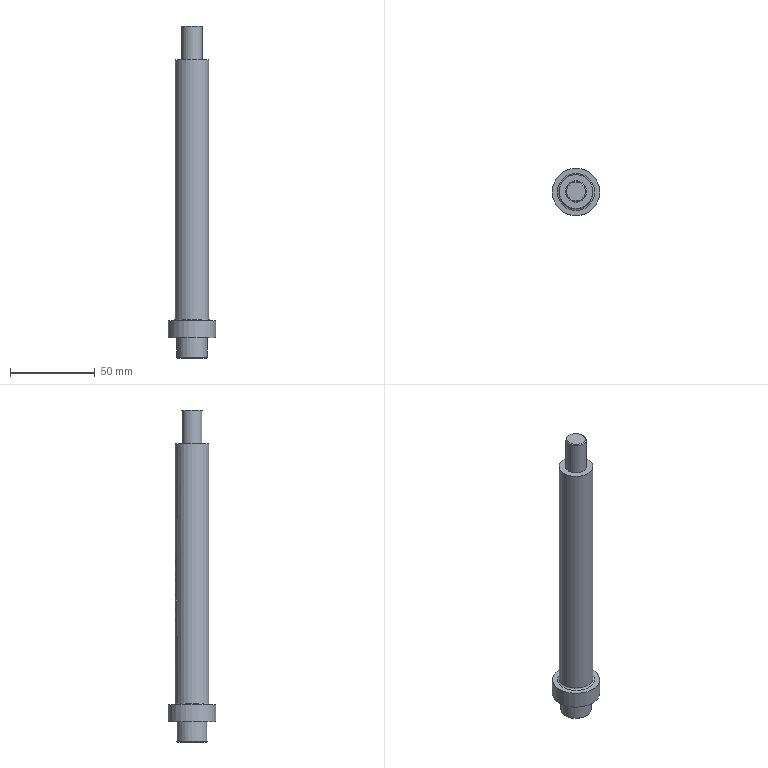Part | NX | features CSR20-100_1 2 | 1 solid | 102 faces | box 28 x 28 x 196 mm | volume 57385 mm3 | plane 55 | cylinder 43 | cone 3 | torus 1 | commonest cylinder face diameters 19.8 x5 20 x3 2.712 x1 2.808 x1 3.225 x1 3.65 x1